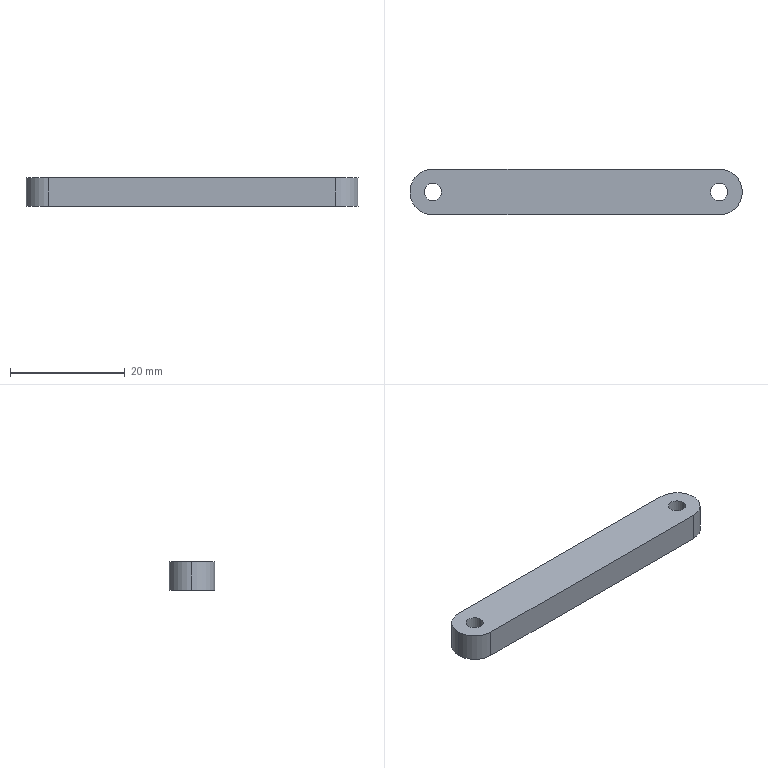Part | SolidWorks | features Extrusion 1, ICE 1 | 1 solid | 11 faces | box 58 x 8 x 5 mm | volume 2181 mm3 | cylinder 7 | plane 4 | commonest cylinder face diameters 3 x4 8 x3
STEP:
#1=CARTESIAN_POINT('',(-26.5,0.,0.));
#2=VERTEX_POINT('',#1);
#3=CARTESIAN_POINT('',(-23.5,0.,0.));
#4=VERTEX_POINT('',#3);
#5=CARTESIAN_POINT('',(-25.,0.,0.));
#6=DIRECTION('',(0.,0.,1.));
#7=DIRECTION('',(1.,0.,0.));
#8=AXIS2_PLACEMENT_3D('',#5,#6,#7);
#9=CIRCLE('',#8,1.5);
#10=EDGE_CURVE('',#2,#4,#9,.T.);
#11=ORIENTED_EDGE('',*,*,#10,.F.);
#12=CARTESIAN_POINT('',(-26.5,0.,5.));
#13=VERTEX_POINT('',#12);
#14=CARTESIAN_POINT('',(-26.5,0.,0.));
#15=DIRECTION('',(0.,0.,1.));
#16=VECTOR('',#15,1000.);
#17=LINE('',#14,#16);
#18=EDGE_CURVE('',#2,#13,#17,.T.);
#19=ORIENTED_EDGE('',*,*,#18,.T.);
#20=CARTESIAN_POINT('',(-23.5,0.,5.));
#21=VERTEX_POINT('',#20);
#22=CARTESIAN_POINT('',(-25.,0.,5.));
#23=DIRECTION('',(0.,0.,1.));
#24=DIRECTION('',(1.,0.,0.));
#25=AXIS2_PLACEMENT_3D('',#22,#23,#24);
#26=CIRCLE('',#25,1.5);
#27=EDGE_CURVE('',#13,#21,#26,.T.);
#28=ORIENTED_EDGE('',*,*,#27,.T.);
#29=CARTESIAN_POINT('',(-23.5,0.,0.));
#30=DIRECTION('',(0.,0.,1.));
#31=VECTOR('',#30,1000.);
#32=LINE('',#29,#31);
#33=EDGE_CURVE('',#4,#21,#32,.T.);
#34=ORIENTED_EDGE('',*,*,#33,.F.);
#35=EDGE_LOOP('',(#11,#19,#28,#34));
#36=FACE_OUTER_BOUND('',#35,.T.);
#37=CARTESIAN_POINT('',(-25.,0.,0.));
#38=DIRECTION('',(0.,0.,1.));
#39=DIRECTION('',(1.,0.,0.));
#40=AXIS2_PLACEMENT_3D('',#37,#38,#39);
#41=CYLINDRICAL_SURFACE('',#40,1.5);
#42=ADVANCED_FACE('',(#36),#41,.F.);
#43=CARTESIAN_POINT('',(23.5,0.,0.));
#44=VERTEX_POINT('',#43);
#45=CARTESIAN_POINT('',(26.5,0.,0.));
#46=VERTEX_POINT('',#45);
#47=CARTESIAN_POINT('',(25.,0.,0.));
#48=DIRECTION('',(0.,0.,1.));
#49=DIRECTION('',(1.,0.,0.));
#50=AXIS2_PLACEMENT_3D('',#47,#48,#49);
#51=CIRCLE('',#50,1.5);
#52=EDGE_CURVE('',#44,#46,#51,.T.);
#53=ORIENTED_EDGE('',*,*,#52,.F.);
#54=CARTESIAN_POINT('',(23.5,0.,5.));
#55=VERTEX_POINT('',#54);
#56=CARTESIAN_POINT('',(23.5,0.,0.));
#57=DIRECTION('',(0.,0.,1.));
#58=VECTOR('',#57,1000.);
#59=LINE('',#56,#58);
#60=EDGE_CURVE('',#44,#55,#59,.T.);
#61=ORIENTED_EDGE('',*,*,#60,.T.);
#62=CARTESIAN_POINT('',(26.5,0.,5.));
#63=VERTEX_POINT('',#62);
#64=CARTESIAN_POINT('',(25.,0.,5.));
#65=DIRECTION('',(0.,0.,1.));
#66=DIRECTION('',(1.,0.,0.));
#67=AXIS2_PLACEMENT_3D('',#64,#65,#66);
#68=CIRCLE('',#67,1.5);
#69=EDGE_CURVE('',#55,#63,#68,.T.);
#70=ORIENTED_EDGE('',*,*,#69,.T.);
#71=CARTESIAN_POINT('',(26.5,0.,0.));
#72=DIRECTION('',(0.,0.,1.));
#73=VECTOR('',#72,1000.);
#74=LINE('',#71,#73);
#75=EDGE_CURVE('',#46,#63,#74,.T.);
#76=ORIENTED_EDGE('',*,*,#75,.F.);
#77=EDGE_LOOP('',(#53,#61,#70,#76));
#78=FACE_OUTER_BOUND('',#77,.T.);
#79=CARTESIAN_POINT('',(25.,0.,0.));
#80=DIRECTION('',(0.,0.,1.));
#81=DIRECTION('',(1.,0.,0.));
#82=AXIS2_PLACEMENT_3D('',#79,#80,#81);
#83=CYLINDRICAL_SURFACE('',#82,1.5);
#84=ADVANCED_FACE('',(#78),#83,.F.);
#85=CARTESIAN_POINT('',(-29.,0.,5.));
#86=VERTEX_POINT('',#85);
#87=CARTESIAN_POINT('',(-25.,-4.,5.));
#88=VERTEX_POINT('',#87);
#89=CARTESIAN_POINT('',(-25.,0.,5.));
#90=DIRECTION('',(0.,0.,1.));
#91=DIRECTION('',(1.,0.,0.));
#92=AXIS2_PLACEMENT_3D('',#89,#90,#91);
#93=CIRCLE('',#92,4.);
#94=EDGE_CURVE('',#86,#88,#93,.T.);
#95=ORIENTED_EDGE('',*,*,#94,.F.);
#96=CARTESIAN_POINT('',(-29.,0.,0.));
#97=VERTEX_POINT('',#96);
#98=CARTESIAN_POINT('',(-29.,0.,5.));
#99=DIRECTION('',(0.,0.,-1.));
#100=VECTOR('',#99,1000.);
#101=LINE('',#98,#100);
#102=EDGE_CURVE('',#86,#97,#101,.T.);
#103=ORIENTED_EDGE('',*,*,#102,.T.);
#104=CARTESIAN_POINT('',(-25.,-4.,0.));
#105=VERTEX_POINT('',#104);
#106=CARTESIAN_POINT('',(-25.,0.,0.));
#107=DIRECTION('',(0.,0.,1.));
#108=DIRECTION('',(1.,0.,0.));
#109=AXIS2_PLACEMENT_3D('',#106,#107,#108);
#110=CIRCLE('',#109,4.);
#111=EDGE_CURVE('',#97,#105,#110,.T.);
#112=ORIENTED_EDGE('',*,*,#111,.T.);
#113=CARTESIAN_POINT('',(-25.,-4.,5.));
#114=DIRECTION('',(0.,0.,-1.));
#115=VECTOR('',#114,1000.);
#116=LINE('',#113,#115);
#117=EDGE_CURVE('',#88,#105,#116,.T.);
#118=ORIENTED_EDGE('',*,*,#117,.F.);
#119=EDGE_LOOP('',(#95,#103,#112,#118));
#120=FACE_OUTER_BOUND('',#119,.T.);
#121=CARTESIAN_POINT('',(-25.,0.,5.));
#122=DIRECTION('',(0.,0.,-1.));
#123=DIRECTION('',(-1.,0.,0.));
#124=AXIS2_PLACEMENT_3D('',#121,#122,#123);
#125=CYLINDRICAL_SURFACE('',#124,4.);
#126=ADVANCED_FACE('',(#120),#125,.T.);
#127=ORIENTED_EDGE('',*,*,#102,.F.);
#128=CARTESIAN_POINT('',(-25.,4.,5.));
#129=VERTEX_POINT('',#128);
#130=CARTESIAN_POINT('',(-25.,0.,5.));
#131=DIRECTION('',(0.,0.,1.));
#132=DIRECTION('',(1.,0.,0.));
#133=AXIS2_PLACEMENT_3D('',#130,#131,#132);
#134=CIRCLE('',#133,4.);
#135=EDGE_CURVE('',#129,#86,#134,.T.);
#136=ORIENTED_EDGE('',*,*,#135,.F.);
#137=CARTESIAN_POINT('',(-25.,4.,0.));
#138=VERTEX_POINT('',#137);
#139=CARTESIAN_POINT('',(-25.,4.,5.));
#140=DIRECTION('',(0.,0.,-1.));
#141=VECTOR('',#140,1000.);
#142=LINE('',#139,#141);
#143=EDGE_CURVE('',#129,#138,#142,.T.);
#144=ORIENTED_EDGE('',*,*,#143,.T.);
#145=CARTESIAN_POINT('',(-25.,0.,0.));
#146=DIRECTION('',(0.,0.,1.));
#147=DIRECTION('',(1.,0.,0.));
#148=AXIS2_PLACEMENT_3D('',#145,#146,#147);
#149=CIRCLE('',#148,4.);
#150=EDGE_CURVE('',#138,#97,#149,.T.);
#151=ORIENTED_EDGE('',*,*,#150,.T.);
#152=EDGE_LOOP('',(#127,#136,#144,#151));
#153=FACE_OUTER_BOUND('',#152,.T.);
#154=CARTESIAN_POINT('',(-25.,0.,5.));
#155=DIRECTION('',(0.,0.,-1.));
#156=DIRECTION('',(-1.,0.,0.));
#157=AXIS2_PLACEMENT_3D('',#154,#155,#156);
#158=CYLINDRICAL_SURFACE('',#157,4.);
#159=ADVANCED_FACE('',(#153),#158,.T.);
#160=CARTESIAN_POINT('',(25.,-4.,0.));
#161=VERTEX_POINT('',#160);
#162=CARTESIAN_POINT('',(-25.,-4.,0.));
#163=DIRECTION('',(1.,0.,0.));
#164=VECTOR('',#163,1000.);
#165=LINE('',#162,#164);
#166=EDGE_CURVE('',#105,#161,#165,.T.);
#167=ORIENTED_EDGE('',*,*,#166,.T.);
#168=CARTESIAN_POINT('',(25.,-4.,5.));
#169=VERTEX_POINT('',#168);
#170=CARTESIAN_POINT('',(25.,-4.,5.));
#171=DIRECTION('',(0.,0.,-1.));
#172=VECTOR('',#171,1000.);
#173=LINE('',#170,#172);
#174=EDGE_CURVE('',#169,#161,#173,.T.);
#175=ORIENTED_EDGE('',*,*,#174,.F.);
#176=CARTESIAN_POINT('',(-25.,-4.,5.));
#177=DIRECTION('',(1.,0.,0.));
#178=VECTOR('',#177,1000.);
#179=LINE('',#176,#178);
#180=EDGE_CURVE('',#88,#169,#179,.T.);
#181=ORIENTED_EDGE('',*,*,#180,.F.);
#182=ORIENTED_EDGE('',*,*,#117,.T.);
#183=EDGE_LOOP('',(#167,#175,#181,#182));
#184=FACE_OUTER_BOUND('',#183,.T.);
#185=CARTESIAN_POINT('',(-25.,-4.,5.));
#186=DIRECTION('',(0.,1.,0.));
#187=DIRECTION('',(0.,0.,1.));
#188=AXIS2_PLACEMENT_3D('',#185,#186,#187);
#189=PLANE('',#188);
#190=ADVANCED_FACE('',(#184),#189,.F.);
#191=CARTESIAN_POINT('',(25.,4.,0.));
#192=VERTEX_POINT('',#191);
#193=CARTESIAN_POINT('',(25.,0.,0.));
#194=DIRECTION('',(0.,0.,1.));
#195=DIRECTION('',(1.,0.,0.));
#196=AXIS2_PLACEMENT_3D('',#193,#194,#195);
#197=CIRCLE('',#196,4.);
#198=EDGE_CURVE('',#161,#192,#197,.T.);
#199=ORIENTED_EDGE('',*,*,#198,.T.);
#200=CARTESIAN_POINT('',(25.,4.,5.));
#201=VERTEX_POINT('',#200);
#202=CARTESIAN_POINT('',(25.,4.,5.));
#203=DIRECTION('',(0.,0.,-1.));
#204=VECTOR('',#203,1000.);
#205=LINE('',#202,#204);
#206=EDGE_CURVE('',#201,#192,#205,.T.);
#207=ORIENTED_EDGE('',*,*,#206,.F.);
#208=CARTESIAN_POINT('',(25.,0.,5.));
#209=DIRECTION('',(0.,0.,1.));
#210=DIRECTION('',(1.,0.,0.));
#211=AXIS2_PLACEMENT_3D('',#208,#209,#210);
#212=CIRCLE('',#211,4.);
#213=EDGE_CURVE('',#169,#201,#212,.T.);
#214=ORIENTED_EDGE('',*,*,#213,.F.);
#215=ORIENTED_EDGE('',*,*,#174,.T.);
#216=EDGE_LOOP('',(#199,#207,#214,#215));
#217=FACE_OUTER_BOUND('',#216,.T.);
#218=CARTESIAN_POINT('',(25.,0.,5.));
#219=DIRECTION('',(0.,0.,-1.));
#220=DIRECTION('',(-1.,0.,0.));
#221=AXIS2_PLACEMENT_3D('',#218,#219,#220);
#222=CYLINDRICAL_SURFACE('',#221,4.);
#223=ADVANCED_FACE('',(#217),#222,.T.);
#224=CARTESIAN_POINT('',(-25.,4.,0.));
#225=DIRECTION('',(-1.,0.,0.));
#226=VECTOR('',#225,1000.);
#227=LINE('',#224,#226);
#228=EDGE_CURVE('',#192,#138,#227,.T.);
#229=ORIENTED_EDGE('',*,*,#228,.T.);
#230=ORIENTED_EDGE('',*,*,#143,.F.);
#231=CARTESIAN_POINT('',(-25.,4.,5.));
#232=DIRECTION('',(-1.,0.,0.));
#233=VECTOR('',#232,1000.);
#234=LINE('',#231,#233);
#235=EDGE_CURVE('',#201,#129,#234,.T.);
#236=ORIENTED_EDGE('',*,*,#235,.F.);
#237=ORIENTED_EDGE('',*,*,#206,.T.);
#238=EDGE_LOOP('',(#229,#230,#236,#237));
#239=FACE_OUTER_BOUND('',#238,.T.);
#240=CARTESIAN_POINT('',(-25.,4.,5.));
#241=DIRECTION('',(0.,-1.,0.));
#242=DIRECTION('',(0.,0.,-1.));
#243=AXIS2_PLACEMENT_3D('',#240,#241,#242);
#244=PLANE('',#243);
#245=ADVANCED_FACE('',(#239),#244,.F.);
#246=CARTESIAN_POINT('',(-25.,0.,5.));
#247=DIRECTION('',(0.,0.,1.));
#248=DIRECTION('',(1.,0.,0.));
#249=AXIS2_PLACEMENT_3D('',#246,#247,#248);
#250=CIRCLE('',#249,1.5);
#251=EDGE_CURVE('',#21,#13,#250,.T.);
#252=ORIENTED_EDGE('',*,*,#251,.F.);
#253=ORIENTED_EDGE('',*,*,#27,.F.);
#254=EDGE_LOOP('',(#252,#253));
#255=FACE_BOUND('',#254,.T.);
#256=CARTESIAN_POINT('',(25.,0.,5.));
#257=DIRECTION('',(0.,0.,1.));
#258=DIRECTION('',(1.,0.,0.));
#259=AXIS2_PLACEMENT_3D('',#256,#257,#258);
#260=CIRCLE('',#259,1.5);
#261=EDGE_CURVE('',#63,#55,#260,.T.);
#262=ORIENTED_EDGE('',*,*,#261,.F.);
#263=ORIENTED_EDGE('',*,*,#69,.F.);
#264=EDGE_LOOP('',(#262,#263));
#265=FACE_BOUND('',#264,.T.);
#266=ORIENTED_EDGE('',*,*,#135,.T.);
#267=ORIENTED_EDGE('',*,*,#94,.T.);
#268=ORIENTED_EDGE('',*,*,#180,.T.);
#269=ORIENTED_EDGE('',*,*,#213,.T.);
#270=ORIENTED_EDGE('',*,*,#235,.T.);
#271=EDGE_LOOP('',(#266,#267,#268,#269,#270));
#272=FACE_OUTER_BOUND('',#271,.T.);
#273=CARTESIAN_POINT('',(-25.,0.,5.));
#274=DIRECTION('',(0.,0.,1.));
#275=DIRECTION('',(1.,0.,0.));
#276=AXIS2_PLACEMENT_3D('',#273,#274,#275);
#277=PLANE('',#276);
#278=ADVANCED_FACE('',(#255,#265,#272),#277,.T.);
#279=CARTESIAN_POINT('',(-25.,0.,0.));
#280=DIRECTION('',(0.,0.,1.));
#281=DIRECTION('',(1.,0.,0.));
#282=AXIS2_PLACEMENT_3D('',#279,#280,#281);
#283=CIRCLE('',#282,1.5);
#284=EDGE_CURVE('',#4,#2,#283,.T.);
#285=ORIENTED_EDGE('',*,*,#284,.T.);
#286=ORIENTED_EDGE('',*,*,#10,.T.);
#287=EDGE_LOOP('',(#285,#286));
#288=FACE_BOUND('',#287,.T.);
#289=CARTESIAN_POINT('',(25.,0.,0.));
#290=DIRECTION('',(0.,0.,1.));
#291=DIRECTION('',(1.,0.,0.));
#292=AXIS2_PLACEMENT_3D('',#289,#290,#291);
#293=CIRCLE('',#292,1.5);
#294=EDGE_CURVE('',#46,#44,#293,.T.);
#295=ORIENTED_EDGE('',*,*,#294,.T.);
#296=ORIENTED_EDGE('',*,*,#52,.T.);
#297=EDGE_LOOP('',(#295,#296));
#298=FACE_BOUND('',#297,.T.);
#299=ORIENTED_EDGE('',*,*,#150,.F.);
#300=ORIENTED_EDGE('',*,*,#228,.F.);
#301=ORIENTED_EDGE('',*,*,#198,.F.);
#302=ORIENTED_EDGE('',*,*,#166,.F.);
#303=ORIENTED_EDGE('',*,*,#111,.F.);
#304=EDGE_LOOP('',(#299,#300,#301,#302,#303));
#305=FACE_OUTER_BOUND('',#304,.T.);
#306=CARTESIAN_POINT('',(-25.,0.,0.));
#307=DIRECTION('',(0.,0.,1.));
#308=DIRECTION('',(1.,0.,0.));
#309=AXIS2_PLACEMENT_3D('',#306,#307,#308);
#310=PLANE('',#309);
#311=ADVANCED_FACE('',(#288,#298,#305),#310,.F.);
#312=ORIENTED_EDGE('',*,*,#60,.F.);
#313=ORIENTED_EDGE('',*,*,#294,.F.);
#314=ORIENTED_EDGE('',*,*,#75,.T.);
#315=ORIENTED_EDGE('',*,*,#261,.T.);
#316=EDGE_LOOP('',(#312,#313,#314,#315));
#317=FACE_OUTER_BOUND('',#316,.T.);
#318=CARTESIAN_POINT('',(25.,0.,0.));
#319=DIRECTION('',(0.,0.,1.));
#320=DIRECTION('',(1.,0.,0.));
#321=AXIS2_PLACEMENT_3D('',#318,#319,#320);
#322=CYLINDRICAL_SURFACE('',#321,1.5);
#323=ADVANCED_FACE('',(#317),#322,.F.);
#324=ORIENTED_EDGE('',*,*,#18,.F.);
#325=ORIENTED_EDGE('',*,*,#284,.F.);
#326=ORIENTED_EDGE('',*,*,#33,.T.);
#327=ORIENTED_EDGE('',*,*,#251,.T.);
#328=EDGE_LOOP('',(#324,#325,#326,#327));
#329=FACE_OUTER_BOUND('',#328,.T.);
#330=CARTESIAN_POINT('',(-25.,0.,0.));
#331=DIRECTION('',(0.,0.,1.));
#332=DIRECTION('',(1.,0.,0.));
#333=AXIS2_PLACEMENT_3D('',#330,#331,#332);
#334=CYLINDRICAL_SURFACE('',#333,1.5);
#335=ADVANCED_FACE('',(#329),#334,.F.);
#336=CLOSED_SHELL('',(#42,#84,#126,#159,#190,#223,#245,#278,#311,#323,#335));
#337=MANIFOLD_SOLID_BREP('',#336);
#338=CARTESIAN_POINT('',(0.,0.,0.));
#339=DIRECTION('',(0.,0.,1.));
#340=DIRECTION('',(1.,0.,0.));
#341=AXIS2_PLACEMENT_3D('',#338,#339,#340);
#342=(LENGTH_UNIT()NAMED_UNIT(*)SI_UNIT(.MILLI.,.METRE.));
#343=UNCERTAINTY_MEASURE_WITH_UNIT(LENGTH_MEASURE(0.00001),#342,'','');
#344=(NAMED_UNIT(*)PLANE_ANGLE_UNIT()SI_UNIT($,.RADIAN.));
#345=(NAMED_UNIT(*)SI_UNIT($,.STERADIAN.)SOLID_ANGLE_UNIT());
#346=(GEOMETRIC_REPRESENTATION_CONTEXT(3)GLOBAL_UNCERTAINTY_ASSIGNED_CONTEXT((#343))GLOBAL_UNIT_ASSIGNED_CONTEXT((#342,#344,#345))REPRESENTATION_CONTEXT('',''));
#347=ADVANCED_BREP_SHAPE_REPRESENTATION('',(#337,#341),#346);